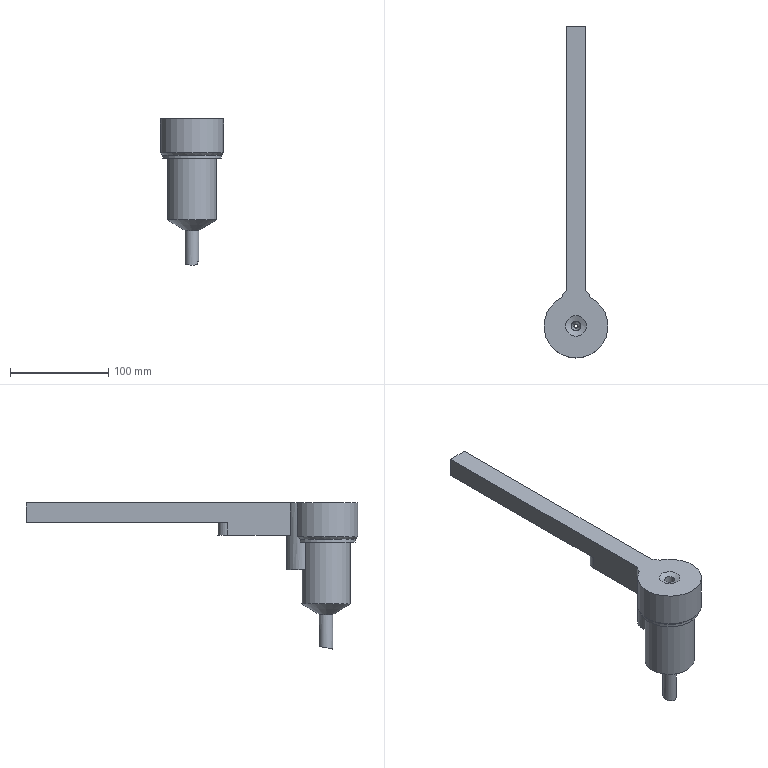Part | STEP file | 车灯-后视镜_id722_x_t | 1 solid | 26 faces | box 65 x 337.5 x 148.701 mm | volume 402158 mm3 | plane 11 | cylinder 7 | cone 4 | sphere 2 | spline 1 | other 1 | commonest cylinder face diameters 10 x1 14 x1 20 x1 30 x1 50 x1 60 x1
STEP:
#1=CARTESIAN_POINT('',(-29.,-25.,97.005));
#2=VERTEX_POINT('',#1);
#3=CARTESIAN_POINT('',(-22.,-25.,97.005));
#4=DIRECTION('',(0.,0.,1.));
#5=DIRECTION('',(-1.,0.,0.));
#6=AXIS2_PLACEMENT_3D('',#3,#4,#5);
#7=CIRCLE('',#6,7.);
#8=EDGE_CURVE('',#2,#2,#7,.T.);
#9=ORIENTED_EDGE('',*,*,#8,.F.);
#10=EDGE_LOOP('',(#9));
#11=FACE_BOUND('',#10,.T.);
#12=CARTESIAN_POINT('',(-15.953,-28.525,62.553));
#13=VERTEX_POINT('',#12);
#14=CARTESIAN_POINT('',(-15.953,-21.475,64.005));
#15=VERTEX_POINT('',#14);
#16=CARTESIAN_POINT('',(-15.953,-28.525,62.553));
#17=CARTESIAN_POINT('',(-16.721,-29.844,62.271));
#18=CARTESIAN_POINT('',(-17.908,-30.885,62.044));
#19=CARTESIAN_POINT('',(-20.758,-32.059,61.786));
#20=CARTESIAN_POINT('',(-22.363,-32.159,61.764));
#21=CARTESIAN_POINT('',(-25.338,-31.343,61.943));
#22=CARTESIAN_POINT('',(-26.657,-30.443,62.141));
#23=CARTESIAN_POINT('',(-28.497,-28.018,62.662));
#24=CARTESIAN_POINT('',(-28.997,-26.523,62.978));
#25=CARTESIAN_POINT('',(-29.003,-23.51,63.598));
#26=CARTESIAN_POINT('',(-28.503,-22.001,63.901));
#27=CARTESIAN_POINT('',(-26.683,-19.581,64.379));
#28=CARTESIAN_POINT('',(-25.346,-18.664,64.556));
#29=CARTESIAN_POINT('',(-22.399,-17.846,64.714));
#30=CARTESIAN_POINT('',(-20.766,-17.942,64.696));
#31=CARTESIAN_POINT('',(-17.938,-19.098,64.472));
#32=CARTESIAN_POINT('',(-16.723,-20.153,64.268));
#33=CARTESIAN_POINT('',(-15.953,-21.475,64.005));
#34=B_SPLINE_CURVE_WITH_KNOTS('',3,(#16,#17,#18,#19,#20,#21,#22,#23,#24,#25,#26,#27,#28,#29,#30,#31,#32,#33),.UNSPECIFIED.,.F.,.F.,(4,2,2,2,2,2,2,2,4),(0.,0.125,0.25,0.375,0.5,0.625,0.75,0.875,1.),.UNSPECIFIED.);
#35=EDGE_CURVE('',#13,#15,#34,.T.);
#36=ORIENTED_EDGE('',*,*,#35,.F.);
#37=CARTESIAN_POINT('',(-15.953,-28.525,65.088));
#38=VERTEX_POINT('',#37);
#39=CARTESIAN_POINT('',(-15.953,-28.525,63.319));
#40=DIRECTION('',(0.,0.,-1.));
#41=VECTOR('',#40,1.);
#42=LINE('',#39,#41);
#43=EDGE_CURVE('',#38,#13,#42,.T.);
#44=ORIENTED_EDGE('',*,*,#43,.F.);
#45=CARTESIAN_POINT('',(-15.953,-21.475,66.533));
#46=VERTEX_POINT('',#45);
#47=CARTESIAN_POINT('',(-15.953,-21.475,66.533));
#48=CARTESIAN_POINT('',(-15.349,-22.51,66.163));
#49=CARTESIAN_POINT('',(-15.009,-23.717,65.827));
#50=CARTESIAN_POINT('',(-14.991,-26.184,65.317));
#51=CARTESIAN_POINT('',(-15.322,-27.443,65.144));
#52=CARTESIAN_POINT('',(-15.953,-28.525,65.088));
#53=B_SPLINE_CURVE_WITH_KNOTS('',3,(#47,#48,#49,#50,#51,#52),.UNSPECIFIED.,.F.,.F.,(4,2,4),(0.,0.5,1.),.UNSPECIFIED.);
#54=EDGE_CURVE('',#46,#38,#53,.T.);
#55=ORIENTED_EDGE('',*,*,#54,.F.);
#56=CARTESIAN_POINT('',(-15.953,-21.475,63.897));
#57=DIRECTION('',(0.,0.,1.));
#58=VECTOR('',#57,1.);
#59=LINE('',#56,#58);
#60=EDGE_CURVE('',#15,#46,#59,.T.);
#61=ORIENTED_EDGE('',*,*,#60,.F.);
#62=EDGE_LOOP('',(#36,#44,#55,#61));
#63=FACE_BOUND('',#62,.T.);
#64=CARTESIAN_POINT('',(-22.,-25.,107.82));
#65=DIRECTION('',(0.,0.,-1.));
#66=DIRECTION('',(1.,0.,0.));
#67=AXIS2_PLACEMENT_3D('',#64,#65,#66);
#68=CYLINDRICAL_SURFACE('',#67,7.);
#69=ADVANCED_FACE('',(#11,#63),#68,.T.);
#70=CARTESIAN_POINT('',(-23.499,-25.,121.));
#71=VERTEX_POINT('',#70);
#72=CARTESIAN_POINT('',(-22.,-25.,121.));
#73=DIRECTION('',(0.,0.,-1.));
#74=DIRECTION('',(-1.,0.,0.));
#75=AXIS2_PLACEMENT_3D('',#72,#73,#74);
#76=CIRCLE('',#75,1.499);
#77=EDGE_CURVE('',#71,#71,#76,.T.);
#78=ORIENTED_EDGE('',*,*,#77,.F.);
#79=EDGE_LOOP('',(#78));
#80=FACE_BOUND('',#79,.T.);
#81=CARTESIAN_POINT('',(-18.452,-27.856,62.695));
#82=VERTEX_POINT('',#81);
#83=CARTESIAN_POINT('',(-18.517,-22.162,63.868));
#84=VERTEX_POINT('',#83);
#85=CARTESIAN_POINT('',(-18.452,-27.856,62.695));
#86=CARTESIAN_POINT('',(-19.029,-28.587,62.54));
#87=CARTESIAN_POINT('',(-19.826,-29.126,62.424));
#88=CARTESIAN_POINT('',(-21.62,-29.654,62.311));
#89=CARTESIAN_POINT('',(-22.603,-29.63,62.316));
#90=CARTESIAN_POINT('',(-24.362,-29.019,62.447));
#91=CARTESIAN_POINT('',(-25.144,-28.43,62.573));
#92=CARTESIAN_POINT('',(-26.213,-26.937,62.889));
#93=CARTESIAN_POINT('',(-26.512,-26.018,63.082));
#94=CARTESIAN_POINT('',(-26.546,-23.28,63.646));
#95=CARTESIAN_POINT('',(-25.348,-21.473,64.006));
#96=CARTESIAN_POINT('',(-21.834,-20.152,64.266));
#97=CARTESIAN_POINT('',(-19.708,-20.724,64.156));
#98=CARTESIAN_POINT('',(-18.517,-22.162,63.868));
#99=B_SPLINE_CURVE_WITH_KNOTS('',3,(#85,#86,#87,#88,#89,#90,#91,#92,#93,#94,#95,#96,#97,#98),.UNSPECIFIED.,.F.,.F.,(4,2,2,2,2,2,4),(0.,0.125,0.25,0.375,0.5,0.75,1.),.UNSPECIFIED.);
#100=EDGE_CURVE('',#82,#84,#99,.T.);
#101=ORIENTED_EDGE('',*,*,#100,.T.);
#102=CARTESIAN_POINT('',(-18.699,-22.21,67.137));
#103=VERTEX_POINT('',#102);
#104=CARTESIAN_POINT('',(-18.517,-22.162,63.868));
#105=CARTESIAN_POINT('',(-18.577,-22.178,64.957));
#106=CARTESIAN_POINT('',(-18.638,-22.194,66.047));
#107=CARTESIAN_POINT('',(-18.699,-22.21,67.137));
#108=B_SPLINE_CURVE_WITH_KNOTS('',3,(#104,#105,#106,#107),.UNSPECIFIED.,.F.,.F.,(4,4),(0.,1.),.UNSPECIFIED.);
#109=EDGE_CURVE('',#84,#103,#108,.T.);
#110=ORIENTED_EDGE('',*,*,#109,.T.);
#111=CARTESIAN_POINT('',(-18.634,-27.807,65.974));
#112=VERTEX_POINT('',#111);
#113=CARTESIAN_POINT('',(-18.699,-22.21,67.137));
#114=CARTESIAN_POINT('',(-18.051,-22.95,66.813));
#115=CARTESIAN_POINT('',(-17.657,-23.933,66.507));
#116=CARTESIAN_POINT('',(-17.611,-25.962,66.079));
#117=CARTESIAN_POINT('',(-17.964,-27.006,65.959));
#118=CARTESIAN_POINT('',(-18.634,-27.807,65.974));
#119=B_SPLINE_CURVE_WITH_KNOTS('',3,(#113,#114,#115,#116,#117,#118),.UNSPECIFIED.,.F.,.F.,(4,2,4),(0.,0.5,1.),.UNSPECIFIED.);
#120=EDGE_CURVE('',#103,#112,#119,.T.);
#121=ORIENTED_EDGE('',*,*,#120,.T.);
#122=CARTESIAN_POINT('',(-18.634,-27.807,65.974));
#123=CARTESIAN_POINT('',(-18.573,-27.823,64.881));
#124=CARTESIAN_POINT('',(-18.512,-27.84,63.788));
#125=CARTESIAN_POINT('',(-18.452,-27.856,62.695));
#126=B_SPLINE_CURVE_WITH_KNOTS('',3,(#122,#123,#124,#125),.UNSPECIFIED.,.F.,.F.,(4,4),(0.,1.),.UNSPECIFIED.);
#127=EDGE_CURVE('',#112,#82,#126,.T.);
#128=ORIENTED_EDGE('',*,*,#127,.T.);
#129=EDGE_LOOP('',(#101,#110,#121,#128));
#130=FACE_BOUND('',#129,.T.);
#131=CARTESIAN_POINT('',(-22.,-25.,120.974));
#132=DIRECTION('',(0.,0.,-1.));
#133=DIRECTION('',(1.,0.,0.));
#134=AXIS2_PLACEMENT_3D('',#131,#132,#133);
#135=CONICAL_SURFACE('',#134,1.501,3.);
#136=ADVANCED_FACE('',(#80,#130),#135,.F.);
#137=CARTESIAN_POINT('',(-12.,75.,190.5));
#138=VERTEX_POINT('',#137);
#139=CARTESIAN_POINT('',(-32.,75.,190.5));
#140=VERTEX_POINT('',#139);
#141=CARTESIAN_POINT('',(-22.,75.,190.5));
#142=DIRECTION('',(0.,0.,1.));
#143=DIRECTION('',(1.,0.,0.));
#144=AXIS2_PLACEMENT_3D('',#141,#142,#143);
#145=CIRCLE('',#144,10.);
#146=EDGE_CURVE('',#138,#140,#145,.T.);
#147=ORIENTED_EDGE('',*,*,#146,.T.);
#148=CARTESIAN_POINT('',(-32.,280.,190.5));
#149=VERTEX_POINT('',#148);
#150=CARTESIAN_POINT('',(-32.,11.18,190.5));
#151=DIRECTION('',(0.,-1.,0.));
#152=VECTOR('',#151,1.);
#153=LINE('',#150,#152);
#154=EDGE_CURVE('',#149,#140,#153,.T.);
#155=ORIENTED_EDGE('',*,*,#154,.F.);
#156=CARTESIAN_POINT('',(-12.,280.,190.5));
#157=VERTEX_POINT('',#156);
#158=CARTESIAN_POINT('',(3.,280.,190.5));
#159=DIRECTION('',(-1.,0.,0.));
#160=VECTOR('',#159,1.);
#161=LINE('',#158,#160);
#162=EDGE_CURVE('',#157,#149,#161,.T.);
#163=ORIENTED_EDGE('',*,*,#162,.F.);
#164=CARTESIAN_POINT('',(-12.,0.,190.5));
#165=DIRECTION('',(0.,-1.,0.));
#166=VECTOR('',#165,1.);
#167=LINE('',#164,#166);
#168=EDGE_CURVE('',#157,#138,#167,.T.);
#169=ORIENTED_EDGE('',*,*,#168,.T.);
#170=EDGE_LOOP('',(#147,#155,#163,#169));
#171=FACE_OUTER_BOUND('',#170,.T.);
#172=CARTESIAN_POINT('',(-22.,0.,190.5));
#173=DIRECTION('',(0.,0.,1.));
#174=DIRECTION('',(0.,-1.,0.));
#175=AXIS2_PLACEMENT_3D('',#172,#173,#174);
#176=PLANE('',#175);
#177=ADVANCED_FACE('',(#171),#176,.F.);
#178=CARTESIAN_POINT('',(-12.,11.18,210.5));
#179=VERTEX_POINT('',#178);
#180=CARTESIAN_POINT('',(-12.,280.,210.5));
#181=VERTEX_POINT('',#180);
#182=CARTESIAN_POINT('',(-12.,11.18,210.5));
#183=DIRECTION('',(0.,1.,0.));
#184=VECTOR('',#183,1.);
#185=LINE('',#182,#184);
#186=EDGE_CURVE('',#179,#181,#185,.T.);
#187=ORIENTED_EDGE('',*,*,#186,.T.);
#188=CARTESIAN_POINT('',(-32.,280.,210.5));
#189=VERTEX_POINT('',#188);
#190=CARTESIAN_POINT('',(3.,280.,210.5));
#191=DIRECTION('',(-1.,0.,0.));
#192=VECTOR('',#191,1.);
#193=LINE('',#190,#192);
#194=EDGE_CURVE('',#181,#189,#193,.T.);
#195=ORIENTED_EDGE('',*,*,#194,.T.);
#196=CARTESIAN_POINT('',(-32.,11.18,210.5));
#197=VERTEX_POINT('',#196);
#198=CARTESIAN_POINT('',(-32.,-25.,210.5));
#199=DIRECTION('',(0.,-1.,0.));
#200=VECTOR('',#199,1.);
#201=LINE('',#198,#200);
#202=EDGE_CURVE('',#189,#197,#201,.T.);
#203=ORIENTED_EDGE('',*,*,#202,.T.);
#204=CARTESIAN_POINT('',(-36.422,4.125,210.5));
#205=VERTEX_POINT('',#204);
#206=CARTESIAN_POINT('',(-22.,0.,210.5));
#207=DIRECTION('',(0.,0.,1.));
#208=DIRECTION('',(1.,0.,0.));
#209=AXIS2_PLACEMENT_3D('',#206,#207,#208);
#210=CIRCLE('',#209,15.);
#211=EDGE_CURVE('',#197,#205,#210,.T.);
#212=ORIENTED_EDGE('',*,*,#211,.T.);
#213=CARTESIAN_POINT('',(-7.578,4.125,210.5));
#214=VERTEX_POINT('',#213);
#215=CARTESIAN_POINT('',(-22.,-25.,210.5));
#216=DIRECTION('',(0.,0.,1.));
#217=DIRECTION('',(1.,0.,0.));
#218=AXIS2_PLACEMENT_3D('',#215,#216,#217);
#219=CIRCLE('',#218,32.5);
#220=EDGE_CURVE('',#205,#214,#219,.T.);
#221=ORIENTED_EDGE('',*,*,#220,.T.);
#222=CARTESIAN_POINT('',(-22.,0.,210.5));
#223=DIRECTION('',(0.,0.,1.));
#224=DIRECTION('',(1.,0.,0.));
#225=AXIS2_PLACEMENT_3D('',#222,#223,#224);
#226=CIRCLE('',#225,15.);
#227=EDGE_CURVE('',#214,#179,#226,.T.);
#228=ORIENTED_EDGE('',*,*,#227,.T.);
#229=EDGE_LOOP('',(#187,#195,#203,#212,#221,#228));
#230=FACE_BOUND('',#229,.T.);
#231=CARTESIAN_POINT('',(-11.464,-25.,210.5));
#232=VERTEX_POINT('',#231);
#233=CARTESIAN_POINT('',(-22.,-25.,210.5));
#234=DIRECTION('',(0.,0.,1.));
#235=DIRECTION('',(1.,0.,0.));
#236=AXIS2_PLACEMENT_3D('',#233,#234,#235);
#237=CIRCLE('',#236,10.536);
#238=EDGE_CURVE('',#232,#232,#237,.T.);
#239=ORIENTED_EDGE('',*,*,#238,.F.);
#240=EDGE_LOOP('',(#239));
#241=FACE_BOUND('',#240,.T.);
#242=CARTESIAN_POINT('',(-22.,-25.,210.5));
#243=DIRECTION('',(0.,0.,1.));
#244=DIRECTION('',(0.,-1.,0.));
#245=AXIS2_PLACEMENT_3D('',#242,#243,#244);
#246=PLANE('',#245);
#247=ADVANCED_FACE('',(#230,#241),#246,.T.);
#248=ORIENTED_EDGE('',*,*,#168,.F.);
#249=CARTESIAN_POINT('',(-12.,280.,0.5));
#250=DIRECTION('',(0.,0.,-1.));
#251=VECTOR('',#250,1.);
#252=LINE('',#249,#251);
#253=EDGE_CURVE('',#181,#157,#252,.T.);
#254=ORIENTED_EDGE('',*,*,#253,.F.);
#255=ORIENTED_EDGE('',*,*,#186,.F.);
#256=CARTESIAN_POINT('',(-12.,11.18,177.5));
#257=VERTEX_POINT('',#256);
#258=CARTESIAN_POINT('',(-12.,11.18,142.5));
#259=DIRECTION('',(0.,0.,1.));
#260=VECTOR('',#259,1.);
#261=LINE('',#258,#260);
#262=EDGE_CURVE('',#257,#179,#261,.T.);
#263=ORIENTED_EDGE('',*,*,#262,.F.);
#264=CARTESIAN_POINT('',(-12.,75.,177.5));
#265=VERTEX_POINT('',#264);
#266=CARTESIAN_POINT('',(-12.,11.18,177.5));
#267=DIRECTION('',(0.,1.,0.));
#268=VECTOR('',#267,1.);
#269=LINE('',#266,#268);
#270=EDGE_CURVE('',#257,#265,#269,.T.);
#271=ORIENTED_EDGE('',*,*,#270,.T.);
#272=CARTESIAN_POINT('',(-12.,75.,162.5));
#273=DIRECTION('',(0.,0.,-1.));
#274=VECTOR('',#273,1.);
#275=LINE('',#272,#274);
#276=EDGE_CURVE('',#138,#265,#275,.T.);
#277=ORIENTED_EDGE('',*,*,#276,.F.);
#278=EDGE_LOOP('',(#248,#254,#255,#263,#271,#277));
#279=FACE_OUTER_BOUND('',#278,.T.);
#280=CARTESIAN_POINT('',(-12.,11.18,172.5));
#281=DIRECTION('',(-1.,0.,0.));
#282=DIRECTION('',(0.,0.,-1.));
#283=AXIS2_PLACEMENT_3D('',#280,#281,#282);
#284=PLANE('',#283);
#285=ADVANCED_FACE('',(#279),#284,.F.);
#286=CARTESIAN_POINT('',(-32.,11.18,177.5));
#287=VERTEX_POINT('',#286);
#288=CARTESIAN_POINT('',(-22.,0.,177.5));
#289=DIRECTION('',(0.,0.,-1.));
#290=DIRECTION('',(1.,0.,0.));
#291=AXIS2_PLACEMENT_3D('',#288,#289,#290);
#292=CIRCLE('',#291,15.);
#293=EDGE_CURVE('',#287,#257,#292,.T.);
#294=ORIENTED_EDGE('',*,*,#293,.F.);
#295=CARTESIAN_POINT('',(-32.,75.,177.5));
#296=VERTEX_POINT('',#295);
#297=CARTESIAN_POINT('',(-32.,11.18,177.5));
#298=DIRECTION('',(0.,1.,0.));
#299=VECTOR('',#298,1.);
#300=LINE('',#297,#299);
#301=EDGE_CURVE('',#287,#296,#300,.T.);
#302=ORIENTED_EDGE('',*,*,#301,.T.);
#303=CARTESIAN_POINT('',(-22.,75.,177.5));
#304=DIRECTION('',(0.,0.,1.));
#305=DIRECTION('',(1.,0.,0.));
#306=AXIS2_PLACEMENT_3D('',#303,#304,#305);
#307=CIRCLE('',#306,10.);
#308=EDGE_CURVE('',#265,#296,#307,.T.);
#309=ORIENTED_EDGE('',*,*,#308,.F.);
#310=ORIENTED_EDGE('',*,*,#270,.F.);
#311=EDGE_LOOP('',(#294,#302,#309,#310));
#312=FACE_OUTER_BOUND('',#311,.T.);
#313=CARTESIAN_POINT('',(-22.,75.,177.5));
#314=DIRECTION('',(0.,0.,1.));
#315=DIRECTION('',(-1.,0.,0.));
#316=AXIS2_PLACEMENT_3D('',#313,#314,#315);
#317=PLANE('',#316);
#318=ADVANCED_FACE('',(#312),#317,.F.);
#319=CARTESIAN_POINT('',(3.,-25.,107.82));
#320=VERTEX_POINT('',#319);
#321=CARTESIAN_POINT('',(-22.,-25.,107.82));
#322=DIRECTION('',(0.,0.,1.));
#323=DIRECTION('',(1.,0.,0.));
#324=AXIS2_PLACEMENT_3D('',#321,#322,#323);
#325=CIRCLE('',#324,25.);
#326=EDGE_CURVE('',#320,#320,#325,.T.);
#327=ORIENTED_EDGE('',*,*,#326,.T.);
#328=EDGE_LOOP('',(#327));
#329=FACE_BOUND('',#328,.T.);
#330=CARTESIAN_POINT('',(-7.691,-4.5,170.5));
#331=VERTEX_POINT('',#330);
#332=CARTESIAN_POINT('',(-36.309,-4.5,170.5));
#333=VERTEX_POINT('',#332);
#334=CARTESIAN_POINT('',(-22.,-25.,170.5));
#335=DIRECTION('',(0.,0.,-1.));
#336=DIRECTION('',(-1.,0.,0.));
#337=AXIS2_PLACEMENT_3D('',#334,#335,#336);
#338=CIRCLE('',#337,25.);
#339=EDGE_CURVE('',#331,#333,#338,.T.);
#340=ORIENTED_EDGE('',*,*,#339,.T.);
#341=CARTESIAN_POINT('',(-36.309,-4.5,142.5));
#342=VERTEX_POINT('',#341);
#343=CARTESIAN_POINT('',(-36.309,-4.5,142.5));
#344=DIRECTION('',(0.,0.,1.));
#345=VECTOR('',#344,1.);
#346=LINE('',#343,#345);
#347=EDGE_CURVE('',#342,#333,#346,.T.);
#348=ORIENTED_EDGE('',*,*,#347,.F.);
#349=CARTESIAN_POINT('',(-7.691,-4.5,142.5));
#350=VERTEX_POINT('',#349);
#351=CARTESIAN_POINT('',(-22.,-25.,142.5));
#352=DIRECTION('',(0.,0.,-1.));
#353=DIRECTION('',(1.,0.,0.));
#354=AXIS2_PLACEMENT_3D('',#351,#352,#353);
#355=CIRCLE('',#354,25.);
#356=EDGE_CURVE('',#342,#350,#355,.T.);
#357=ORIENTED_EDGE('',*,*,#356,.T.);
#358=CARTESIAN_POINT('',(-7.691,-4.5,-145.68));
#359=DIRECTION('',(0.,0.,-1.));
#360=VECTOR('',#359,1.);
#361=LINE('',#358,#360);
#362=EDGE_CURVE('',#331,#350,#361,.T.);
#363=ORIENTED_EDGE('',*,*,#362,.F.);
#364=EDGE_LOOP('',(#340,#348,#357,#363));
#365=FACE_BOUND('',#364,.T.);
#366=CARTESIAN_POINT('',(-22.,-25.,-145.68));
#367=DIRECTION('',(0.,0.,1.));
#368=DIRECTION('',(-1.,0.,0.));
#369=AXIS2_PLACEMENT_3D('',#366,#367,#368);
#370=CYLINDRICAL_SURFACE('',#369,25.);
#371=ADVANCED_FACE('',(#329,#365),#370,.T.);
#372=CARTESIAN_POINT('',(-22.,0.,142.5));
#373=DIRECTION('',(0.,0.,-1.));
#374=DIRECTION('',(1.,0.,0.));
#375=AXIS2_PLACEMENT_3D('',#372,#373,#374);
#376=CIRCLE('',#375,15.);
#377=EDGE_CURVE('',#342,#350,#376,.T.);
#378=ORIENTED_EDGE('',*,*,#377,.F.);
#379=ORIENTED_EDGE('',*,*,#347,.T.);
#380=CARTESIAN_POINT('',(-36.967,1.,170.5));
#381=VERTEX_POINT('',#380);
#382=CARTESIAN_POINT('',(-22.,0.,170.5));
#383=DIRECTION('',(0.,0.,-1.));
#384=DIRECTION('',(-1.,0.,0.));
#385=AXIS2_PLACEMENT_3D('',#382,#383,#384);
#386=CIRCLE('',#385,15.);
#387=EDGE_CURVE('',#333,#381,#386,.T.);
#388=ORIENTED_EDGE('',*,*,#387,.T.);
#389=CARTESIAN_POINT('',(-36.967,1.,173.5));
#390=VERTEX_POINT('',#389);
#391=CARTESIAN_POINT('',(-36.967,1.,186.5));
#392=DIRECTION('',(0.,0.,1.));
#393=VECTOR('',#392,1.);
#394=LINE('',#391,#393);
#395=EDGE_CURVE('',#381,#390,#394,.T.);
#396=ORIENTED_EDGE('',*,*,#395,.T.);
#397=CARTESIAN_POINT('',(-36.422,4.125,176.));
#398=VERTEX_POINT('',#397);
#399=CARTESIAN_POINT('',(-36.967,1.,173.5));
#400=CARTESIAN_POINT('',(-36.932,1.518,173.931));
#401=CARTESIAN_POINT('',(-36.87,2.042,174.359));
#402=CARTESIAN_POINT('',(-36.689,3.085,175.193));
#403=CARTESIAN_POINT('',(-36.57,3.606,175.601));
#404=CARTESIAN_POINT('',(-36.422,4.125,176.));
#405=B_SPLINE_CURVE_WITH_KNOTS('',3,(#399,#400,#401,#402,#403,#404),.UNSPECIFIED.,.F.,.F.,(4,2,4),(0.,0.5,1.),.UNSPECIFIED.);
#406=EDGE_CURVE('',#390,#398,#405,.T.);
#407=ORIENTED_EDGE('',*,*,#406,.T.);
#408=CARTESIAN_POINT('',(-36.422,4.125,186.5));
#409=DIRECTION('',(0.,0.,1.));
#410=VECTOR('',#409,1.);
#411=LINE('',#408,#410);
#412=EDGE_CURVE('',#398,#205,#411,.T.);
#413=ORIENTED_EDGE('',*,*,#412,.T.);
#414=ORIENTED_EDGE('',*,*,#211,.F.);
#415=CARTESIAN_POINT('',(-32.,11.18,142.5));
#416=DIRECTION('',(0.,0.,1.));
#417=VECTOR('',#416,1.);
#418=LINE('',#415,#417);
#419=EDGE_CURVE('',#287,#197,#418,.T.);
#420=ORIENTED_EDGE('',*,*,#419,.F.);
#421=ORIENTED_EDGE('',*,*,#293,.T.);
#422=ORIENTED_EDGE('',*,*,#262,.T.);
#423=ORIENTED_EDGE('',*,*,#227,.F.);
#424=CARTESIAN_POINT('',(-7.578,4.125,176.));
#425=VERTEX_POINT('',#424);
#426=CARTESIAN_POINT('',(-7.578,4.125,186.5));
#427=DIRECTION('',(0.,0.,-1.));
#428=VECTOR('',#427,1.);
#429=LINE('',#426,#428);
#430=EDGE_CURVE('',#214,#425,#429,.T.);
#431=ORIENTED_EDGE('',*,*,#430,.T.);
#432=CARTESIAN_POINT('',(-7.033,1.,173.5));
#433=VERTEX_POINT('',#432);
#434=CARTESIAN_POINT('',(-7.578,4.125,176.));
#435=CARTESIAN_POINT('',(-7.43,3.606,175.601));
#436=CARTESIAN_POINT('',(-7.311,3.085,175.192));
#437=CARTESIAN_POINT('',(-7.129,2.037,174.355));
#438=CARTESIAN_POINT('',(-7.068,1.514,173.929));
#439=CARTESIAN_POINT('',(-7.033,1.,173.5));
#440=B_SPLINE_CURVE_WITH_KNOTS('',3,(#434,#435,#436,#437,#438,#439),.UNSPECIFIED.,.F.,.F.,(4,2,4),(0.,0.5,1.),.UNSPECIFIED.);
#441=EDGE_CURVE('',#425,#433,#440,.T.);
#442=ORIENTED_EDGE('',*,*,#441,.T.);
#443=CARTESIAN_POINT('',(-7.033,1.,170.5));
#444=VERTEX_POINT('',#443);
#445=CARTESIAN_POINT('',(-7.033,1.,186.5));
#446=DIRECTION('',(0.,0.,-1.));
#447=VECTOR('',#446,1.);
#448=LINE('',#445,#447);
#449=EDGE_CURVE('',#433,#444,#448,.T.);
#450=ORIENTED_EDGE('',*,*,#449,.T.);
#451=CARTESIAN_POINT('',(-22.,0.,170.5));
#452=DIRECTION('',(0.,0.,-1.));
#453=DIRECTION('',(-1.,0.,0.));
#454=AXIS2_PLACEMENT_3D('',#451,#452,#453);
#455=CIRCLE('',#454,15.);
#456=EDGE_CURVE('',#444,#331,#455,.T.);
#457=ORIENTED_EDGE('',*,*,#456,.T.);
#458=ORIENTED_EDGE('',*,*,#362,.T.);
#459=EDGE_LOOP('',(#378,#379,#388,#396,#407,#413,#414,#420,#421,#422,#423,#431,#442,#450,#457,#458));
#460=FACE_OUTER_BOUND('',#459,.T.);
#461=CARTESIAN_POINT('',(-22.,0.,142.5));
#462=DIRECTION('',(0.,0.,1.));
#463=DIRECTION('',(-1.,0.,0.));
#464=AXIS2_PLACEMENT_3D('',#461,#462,#463);
#465=CYLINDRICAL_SURFACE('',#464,15.);
#466=ADVANCED_FACE('',(#460),#465,.T.);
#467=ORIENTED_EDGE('',*,*,#356,.F.);
#468=ORIENTED_EDGE('',*,*,#377,.T.);
#469=EDGE_LOOP('',(#467,#468));
#470=FACE_OUTER_BOUND('',#469,.T.);
#471=CARTESIAN_POINT('',(-19.,-12.5,142.5));
#472=DIRECTION('',(0.,0.,1.));
#473=DIRECTION('',(-1.,0.,0.));
#474=AXIS2_PLACEMENT_3D('',#471,#472,#473);
#475=PLANE('',#474);
#476=ADVANCED_FACE('',(#470),#475,.F.);
#477=ORIENTED_EDGE('',*,*,#8,.T.);
#478=EDGE_LOOP('',(#477));
#479=FACE_BOUND('',#478,.T.);
#480=ORIENTED_EDGE('',*,*,#326,.F.);
#481=EDGE_LOOP('',(#480));
#482=FACE_BOUND('',#481,.T.);
#483=CARTESIAN_POINT('',(-22.,-25.,92.798));
#484=DIRECTION('',(0.,0.,1.));
#485=DIRECTION('',(-1.,0.,0.));
#486=AXIS2_PLACEMENT_3D('',#483,#484,#485);
#487=CONICAL_SURFACE('',#486,0.,59.);
#488=ADVANCED_FACE('',(#479,#482),#487,.T.);
#489=ORIENTED_EDGE('',*,*,#220,.F.);
#490=ORIENTED_EDGE('',*,*,#412,.F.);
#491=CARTESIAN_POINT('',(-22.,-25.,176.));
#492=DIRECTION('',(0.,0.,1.));
#493=DIRECTION('',(1.,0.,0.));
#494=AXIS2_PLACEMENT_3D('',#491,#492,#493);
#495=CIRCLE('',#494,32.5);
#496=EDGE_CURVE('',#398,#425,#495,.T.);
#497=ORIENTED_EDGE('',*,*,#496,.T.);
#498=ORIENTED_EDGE('',*,*,#430,.F.);
#499=EDGE_LOOP('',(#489,#490,#497,#498));
#500=FACE_OUTER_BOUND('',#499,.T.);
#501=CARTESIAN_POINT('',(-22.,-25.,210.5));
#502=DIRECTION('',(0.,0.,-1.));
#503=DIRECTION('',(1.,0.,0.));
#504=AXIS2_PLACEMENT_3D('',#501,#502,#503);
#505=CYLINDRICAL_SURFACE('',#504,32.5);
#506=ADVANCED_FACE('',(#500),#505,.T.);
#507=ORIENTED_EDGE('',*,*,#496,.F.);
#508=ORIENTED_EDGE('',*,*,#406,.F.);
#509=CARTESIAN_POINT('',(-22.,-25.,173.5));
#510=DIRECTION('',(0.,0.,1.));
#511=DIRECTION('',(-1.,0.,0.));
#512=AXIS2_PLACEMENT_3D('',#509,#510,#511);
#513=CIRCLE('',#512,30.);
#514=EDGE_CURVE('',#390,#433,#513,.T.);
#515=ORIENTED_EDGE('',*,*,#514,.T.);
#516=ORIENTED_EDGE('',*,*,#441,.F.);
#517=EDGE_LOOP('',(#507,#508,#515,#516));
#518=FACE_OUTER_BOUND('',#517,.T.);
#519=CARTESIAN_POINT('',(-22.,-25.,176.));
#520=DIRECTION('',(0.,0.,1.));
#521=DIRECTION('',(1.,0.,0.));
#522=AXIS2_PLACEMENT_3D('',#519,#520,#521);
#523=CONICAL_SURFACE('',#522,32.5,45.);
#524=ADVANCED_FACE('',(#518),#523,.T.);
#525=ORIENTED_EDGE('',*,*,#514,.F.);
#526=ORIENTED_EDGE('',*,*,#395,.F.);
#527=CARTESIAN_POINT('',(-22.,-25.,170.5));
#528=DIRECTION('',(0.,0.,-1.));
#529=DIRECTION('',(-1.,0.,0.));
#530=AXIS2_PLACEMENT_3D('',#527,#528,#529);
#531=CIRCLE('',#530,30.);
#532=EDGE_CURVE('',#444,#381,#531,.T.);
#533=ORIENTED_EDGE('',*,*,#532,.F.);
#534=ORIENTED_EDGE('',*,*,#449,.F.);
#535=EDGE_LOOP('',(#525,#526,#533,#534));
#536=FACE_OUTER_BOUND('',#535,.T.);
#537=CARTESIAN_POINT('',(-22.,-25.,176.));
#538=DIRECTION('',(0.,0.,-1.));
#539=DIRECTION('',(1.,0.,0.));
#540=AXIS2_PLACEMENT_3D('',#537,#538,#539);
#541=CYLINDRICAL_SURFACE('',#540,30.);
#542=ADVANCED_FACE('',(#536),#541,.T.);
#543=ORIENTED_EDGE('',*,*,#532,.T.);
#544=ORIENTED_EDGE('',*,*,#387,.F.);
#545=ORIENTED_EDGE('',*,*,#339,.F.);
#546=ORIENTED_EDGE('',*,*,#456,.F.);
#547=EDGE_LOOP('',(#543,#544,#545,#546));
#548=FACE_OUTER_BOUND('',#547,.T.);
#549=CARTESIAN_POINT('',(-22.,-25.,170.5));
#550=DIRECTION('',(0.,0.,-1.));
#551=DIRECTION('',(1.,0.,0.));
#552=AXIS2_PLACEMENT_3D('',#549,#550,#551);
#553=PLANE('',#552);
#554=ADVANCED_FACE('',(#548),#553,.T.);
#555=ORIENTED_EDGE('',*,*,#308,.T.);
#556=CARTESIAN_POINT('',(-32.,75.,172.5));
#557=DIRECTION('',(0.,0.,1.));
#558=VECTOR('',#557,1.);
#559=LINE('',#556,#558);
#560=EDGE_CURVE('',#296,#140,#559,.T.);
#561=ORIENTED_EDGE('',*,*,#560,.T.);
#562=ORIENTED_EDGE('',*,*,#146,.F.);
#563=ORIENTED_EDGE('',*,*,#276,.T.);
#564=EDGE_LOOP('',(#555,#561,#562,#563));
#565=FACE_OUTER_BOUND('',#564,.T.);
#566=CARTESIAN_POINT('',(-22.,75.,172.5));
#567=DIRECTION('',(0.,0.,-1.));
#568=DIRECTION('',(0.,1.,0.));
#569=AXIS2_PLACEMENT_3D('',#566,#567,#568);
#570=CYLINDRICAL_SURFACE('',#569,10.);
#571=ADVANCED_FACE('',(#565),#570,.T.);
#572=ORIENTED_EDGE('',*,*,#238,.T.);
#573=EDGE_LOOP('',(#572));
#574=FACE_BOUND('',#573,.T.);
#575=CARTESIAN_POINT('',(-17.,-25.,208.135));
#576=VERTEX_POINT('',#575);
#577=CARTESIAN_POINT('',(-22.,-25.,208.135));
#578=DIRECTION('',(0.,0.,1.));
#579=DIRECTION('',(1.,0.,0.));
#580=AXIS2_PLACEMENT_3D('',#577,#578,#579);
#581=CIRCLE('',#580,5.);
#582=EDGE_CURVE('',#576,#576,#581,.T.);
#583=ORIENTED_EDGE('',*,*,#582,.F.);
#584=EDGE_LOOP('',(#583));
#585=FACE_BOUND('',#584,.T.);
#586=CARTESIAN_POINT('',(-22.,-25.,227.5));
#587=DIRECTION('',(0.,0.,1.));
#588=DIRECTION('',(1.,0.,0.));
#589=AXIS2_PLACEMENT_3D('',#586,#587,#588);
#590=SPHERICAL_SURFACE('',#589,20.);
#591=ADVANCED_FACE('',(#574,#585),#590,.F.);
#592=CARTESIAN_POINT('',(-19.599,-25.,121.));
#593=VERTEX_POINT('',#592);
#594=CARTESIAN_POINT('',(-22.,-25.,121.));
#595=DIRECTION('',(0.,0.,-1.));
#596=DIRECTION('',(1.,0.,0.));
#597=AXIS2_PLACEMENT_3D('',#594,#595,#596);
#598=CIRCLE('',#597,2.401);
#599=EDGE_CURVE('',#593,#593,#598,.T.);
#600=ORIENTED_EDGE('',*,*,#599,.F.);
#601=EDGE_LOOP('',(#600));
#602=FACE_BOUND('',#601,.T.);
#603=ORIENTED_EDGE('',*,*,#77,.T.);
#604=EDGE_LOOP('',(#603));
#605=FACE_BOUND('',#604,.T.);
#606=CARTESIAN_POINT('',(-22.,-25.,121.));
#607=DIRECTION('',(0.,0.,-1.));
#608=DIRECTION('',(1.,0.,0.));
#609=AXIS2_PLACEMENT_3D('',#606,#607,#608);
#610=PLANE('',#609);
#611=ADVANCED_FACE('',(#602,#605),#610,.F.);
#612=ORIENTED_EDGE('',*,*,#202,.F.);
#613=CARTESIAN_POINT('',(-32.,280.,0.5));
#614=DIRECTION('',(0.,0.,-1.));
#615=VECTOR('',#614,1.);
#616=LINE('',#613,#615);
#617=EDGE_CURVE('',#189,#149,#616,.T.);
#618=ORIENTED_EDGE('',*,*,#617,.T.);
#619=ORIENTED_EDGE('',*,*,#154,.T.);
#620=ORIENTED_EDGE('',*,*,#560,.F.);
#621=ORIENTED_EDGE('',*,*,#301,.F.);
#622=ORIENTED_EDGE('',*,*,#419,.T.);
#623=EDGE_LOOP('',(#612,#618,#619,#620,#621,#622));
#624=FACE_OUTER_BOUND('',#623,.T.);
#625=CARTESIAN_POINT('',(-32.,11.18,172.5));
#626=DIRECTION('',(-1.,0.,0.));
#627=DIRECTION('',(0.,1.,0.));
#628=AXIS2_PLACEMENT_3D('',#625,#626,#627);
#629=PLANE('',#628);
#630=ADVANCED_FACE('',(#624),#629,.T.);
#631=CARTESIAN_POINT('',(-27.,-25.,129.792));
#632=VERTEX_POINT('',#631);
#633=CARTESIAN_POINT('',(-22.,-25.,129.792));
#634=DIRECTION('',(0.,0.,1.));
#635=DIRECTION('',(-1.,0.,0.));
#636=AXIS2_PLACEMENT_3D('',#633,#634,#635);
#637=CIRCLE('',#636,5.);
#638=EDGE_CURVE('',#632,#632,#637,.T.);
#639=ORIENTED_EDGE('',*,*,#638,.F.);
#640=EDGE_LOOP('',(#639));
#641=FACE_BOUND('',#640,.T.);
#642=ORIENTED_EDGE('',*,*,#582,.T.);
#643=EDGE_LOOP('',(#642));
#644=FACE_BOUND('',#643,.T.);
#645=CARTESIAN_POINT('',(-22.,-25.,99.5));
#646=DIRECTION('',(0.,0.,1.));
#647=DIRECTION('',(-1.,0.,0.));
#648=AXIS2_PLACEMENT_3D('',#645,#646,#647);
#649=CYLINDRICAL_SURFACE('',#648,5.);
#650=ADVANCED_FACE('',(#641,#644),#649,.F.);
#651=CARTESIAN_POINT('',(-26.755,-25.,128.247));
#652=VERTEX_POINT('',#651);
#653=CARTESIAN_POINT('',(-22.,-25.,128.247));
#654=DIRECTION('',(0.,0.,-1.));
#655=DIRECTION('',(-1.,0.,0.));
#656=AXIS2_PLACEMENT_3D('',#653,#654,#655);
#657=CIRCLE('',#656,4.755);
#658=EDGE_CURVE('',#652,#652,#657,.T.);
#659=ORIENTED_EDGE('',*,*,#658,.F.);
#660=EDGE_LOOP('',(#659));
#661=FACE_BOUND('',#660,.T.);
#662=ORIENTED_EDGE('',*,*,#599,.T.);
#663=EDGE_LOOP('',(#662));
#664=FACE_BOUND('',#663,.T.);
#665=CARTESIAN_POINT('',(-22.,-25.,129.));
#666=DIRECTION('',(0.,0.,1.));
#667=DIRECTION('',(-1.,0.,0.));
#668=AXIS2_PLACEMENT_3D('',#665,#666,#667);
#669=CONICAL_SURFACE('',#668,5.,18.);
#670=ADVANCED_FACE('',(#661,#664),#669,.F.);
#671=ORIENTED_EDGE('',*,*,#638,.T.);
#672=EDGE_LOOP('',(#671));
#673=FACE_BOUND('',#672,.T.);
#674=ORIENTED_EDGE('',*,*,#658,.T.);
#675=EDGE_LOOP('',(#674));
#676=FACE_BOUND('',#675,.T.);
#677=CARTESIAN_POINT('',(-22.,-25.,129.792));
#678=DIRECTION('',(0.,0.,1.));
#679=DIRECTION('',(-1.,0.,0.));
#680=AXIS2_PLACEMENT_3D('',#677,#678,#679);
#681=SPHERICAL_SURFACE('',#680,5.);
#682=ADVANCED_FACE('',(#673,#676),#681,.F.);
#683=ORIENTED_EDGE('',*,*,#253,.T.);
#684=ORIENTED_EDGE('',*,*,#162,.T.);
#685=ORIENTED_EDGE('',*,*,#617,.F.);
#686=ORIENTED_EDGE('',*,*,#194,.F.);
#687=EDGE_LOOP('',(#683,#684,#685,#686));
#688=FACE_OUTER_BOUND('',#687,.T.);
#689=CARTESIAN_POINT('',(3.,280.,0.5));
#690=DIRECTION('',(0.,1.,0.));
#691=DIRECTION('',(0.,0.,1.));
#692=AXIS2_PLACEMENT_3D('',#689,#690,#691);
#693=PLANE('',#692);
#694=ADVANCED_FACE('',(#688),#693,.T.);
#695=ORIENTED_EDGE('',*,*,#43,.T.);
#696=CARTESIAN_POINT('',(-18.452,-27.856,62.695));
#697=CARTESIAN_POINT('',(-17.619,-28.079,62.648));
#698=CARTESIAN_POINT('',(-16.786,-28.302,62.6));
#699=CARTESIAN_POINT('',(-15.953,-28.525,62.553));
#700=B_SPLINE_CURVE_WITH_KNOTS('',3,(#696,#697,#698,#699),.UNSPECIFIED.,.F.,.F.,(4,4),(0.,1.),.UNSPECIFIED.);
#701=EDGE_CURVE('',#82,#13,#700,.T.);
#702=ORIENTED_EDGE('',*,*,#701,.F.);
#703=ORIENTED_EDGE('',*,*,#127,.F.);
#704=CARTESIAN_POINT('',(-15.953,-28.525,65.088));
#705=CARTESIAN_POINT('',(-16.846,-28.286,65.383));
#706=CARTESIAN_POINT('',(-17.74,-28.047,65.678));
#707=CARTESIAN_POINT('',(-18.634,-27.807,65.974));
#708=B_SPLINE_CURVE_WITH_KNOTS('',3,(#704,#705,#706,#707),.UNSPECIFIED.,.F.,.F.,(4,4),(0.,1.),.UNSPECIFIED.);
#709=EDGE_CURVE('',#38,#112,#708,.T.);
#710=ORIENTED_EDGE('',*,*,#709,.F.);
#711=EDGE_LOOP('',(#695,#702,#703,#710));
#712=FACE_OUTER_BOUND('',#711,.T.);
#713=CARTESIAN_POINT('',(-12.316,-29.5,61.427));
#714=DIRECTION('',(-0.2588,-0.9659,0.));
#715=DIRECTION('',(0.9659,-0.2588,0.));
#716=AXIS2_PLACEMENT_3D('',#713,#714,#715);
#717=PLANE('',#716);
#718=ADVANCED_FACE('',(#712),#717,.F.);
#719=ORIENTED_EDGE('',*,*,#54,.T.);
#720=ORIENTED_EDGE('',*,*,#709,.T.);
#721=ORIENTED_EDGE('',*,*,#120,.F.);
#722=CARTESIAN_POINT('',(-18.699,-22.21,67.137));
#723=CARTESIAN_POINT('',(-17.783,-21.965,66.936));
#724=CARTESIAN_POINT('',(-16.868,-21.72,66.734));
#725=CARTESIAN_POINT('',(-15.953,-21.475,66.533));
#726=B_SPLINE_CURVE_WITH_KNOTS('',3,(#722,#723,#724,#725),.UNSPECIFIED.,.F.,.F.,(4,4),(0.,1.),.UNSPECIFIED.);
#727=EDGE_CURVE('',#103,#46,#726,.T.);
#728=ORIENTED_EDGE('',*,*,#727,.T.);
#729=EDGE_LOOP('',(#719,#720,#721,#728));
#730=FACE_OUTER_BOUND('',#729,.T.);
#731=CARTESIAN_POINT('',(-21.316,36.979,76.906));
#732=CARTESIAN_POINT('',(-21.316,22.634,75.233));
#733=CARTESIAN_POINT('',(-21.316,8.315,73.269));
#734=CARTESIAN_POINT('',(-21.316,-20.212,68.418));
#735=CARTESIAN_POINT('',(-21.316,-34.398,65.517));
#736=CARTESIAN_POINT('',(-21.316,-48.448,61.901));
#737=CARTESIAN_POINT('',(-9.316,37.352,73.712));
#738=CARTESIAN_POINT('',(-9.316,23.052,72.045));
#739=CARTESIAN_POINT('',(-9.316,8.785,70.087));
#740=CARTESIAN_POINT('',(-9.316,-19.603,65.26));
#741=CARTESIAN_POINT('',(-9.316,-33.7,62.376));
#742=CARTESIAN_POINT('',(-9.316,-47.646,58.787));
#743=B_SPLINE_SURFACE_WITH_KNOTS('',1,3,((#731,#732,#733,#734,#735,#736),(#737,#738,#739,#740,#741,#742)),.UNSPECIFIED.,.F.,.F.,.F.,(2,2),(4,2,4),(0.,1.),(0.,0.5,1.),.UNSPECIFIED.);
#744=ADVANCED_FACE('',(#730),#743,.T.);
#745=ORIENTED_EDGE('',*,*,#60,.T.);
#746=ORIENTED_EDGE('',*,*,#727,.F.);
#747=ORIENTED_EDGE('',*,*,#109,.F.);
#748=CARTESIAN_POINT('',(-15.953,-21.475,64.005));
#749=CARTESIAN_POINT('',(-16.807,-21.704,63.959));
#750=CARTESIAN_POINT('',(-17.662,-21.933,63.914));
#751=CARTESIAN_POINT('',(-18.517,-22.162,63.868));
#752=B_SPLINE_CURVE_WITH_KNOTS('',3,(#748,#749,#750,#751),.UNSPECIFIED.,.F.,.F.,(4,4),(0.,1.),.UNSPECIFIED.);
#753=EDGE_CURVE('',#15,#84,#752,.T.);
#754=ORIENTED_EDGE('',*,*,#753,.F.);
#755=EDGE_LOOP('',(#745,#746,#747,#754));
#756=FACE_OUTER_BOUND('',#755,.T.);
#757=CARTESIAN_POINT('',(-12.316,-20.5,62.147));
#758=DIRECTION('',(-0.2588,0.9659,0.));
#759=DIRECTION('',(-0.9659,-0.2588,0.));
#760=AXIS2_PLACEMENT_3D('',#757,#758,#759);
#761=PLANE('',#760);
#762=ADVANCED_FACE('',(#756),#761,.F.);
#763=ORIENTED_EDGE('',*,*,#701,.T.);
#764=ORIENTED_EDGE('',*,*,#35,.T.);
#765=ORIENTED_EDGE('',*,*,#753,.T.);
#766=ORIENTED_EDGE('',*,*,#100,.F.);
#767=EDGE_LOOP('',(#763,#764,#765,#766));
#768=FACE_OUTER_BOUND('',#767,.T.);
#769=CARTESIAN_POINT('',(-12.332,37.444,73.018));
#770=CARTESIAN_POINT('',(-12.381,30.166,72.169));
#771=CARTESIAN_POINT('',(-12.445,22.978,71.252));
#772=CARTESIAN_POINT('',(-12.521,15.838,70.249));
#773=CARTESIAN_POINT('',(-12.596,8.698,69.246));
#774=CARTESIAN_POINT('',(-12.683,1.606,68.157));
#775=CARTESIAN_POINT('',(-12.783,-5.456,66.954));
#776=CARTESIAN_POINT('',(-12.883,-12.518,65.751));
#777=CARTESIAN_POINT('',(-12.995,-19.549,64.434));
#778=CARTESIAN_POINT('',(-13.126,-26.549,62.97));
#779=CARTESIAN_POINT('',(-13.256,-33.549,61.506));
#780=CARTESIAN_POINT('',(-13.404,-40.518,59.896));
#781=CARTESIAN_POINT('',(-13.579,-47.447,58.113));
#782=B_SPLINE_CURVE_WITH_KNOTS('',3,(#769,#770,#771,#772,#773,#774,#775,#776,#777,#778,#779,#780,#781),.UNSPECIFIED.,.F.,.F.,(4,3,3,3,4),(0.,0.25,0.5,0.75,1.),.UNSPECIFIED.);
#783=DIRECTION('',(-1.,0.,0.));
#784=VECTOR('',#783,1.);
#785=SURFACE_OF_LINEAR_EXTRUSION('',#782,#784);
#786=ADVANCED_FACE('',(#768),#785,.T.);
#787=CLOSED_SHELL('',(#69,#136,#177,#247,#285,#318,#371,#466,#476,#488,#506,#524,#542,#554,#571,#591,#611,#630,#650,#670,#682,#694,#718,#744,#762,#786));
#788=MANIFOLD_SOLID_BREP('',#787);
#789=(LENGTH_UNIT()NAMED_UNIT(*)SI_UNIT(.MILLI.,.METRE.));
#790=UNCERTAINTY_MEASURE_WITH_UNIT(LENGTH_MEASURE(0.0508),#789,'','');
#791=(NAMED_UNIT(*)PLANE_ANGLE_UNIT()SI_UNIT($,.RADIAN.));
#792=PLANE_ANGLE_MEASURE_WITH_UNIT(PLANE_ANGLE_MEASURE(0.01745),#791);
#793=DIMENSIONAL_EXPONENTS(0.,0.,0.,0.,0.,0.,0.);
#794=(CONVERSION_BASED_UNIT('DEGREE',#792)NAMED_UNIT(#793)PLANE_ANGLE_UNIT());
#795=(NAMED_UNIT(*)SI_UNIT($,.STERADIAN.)SOLID_ANGLE_UNIT());
#796=(GEOMETRIC_REPRESENTATION_CONTEXT(3)GLOBAL_UNCERTAINTY_ASSIGNED_CONTEXT((#790))GLOBAL_UNIT_ASSIGNED_CONTEXT((#789,#794,#795))REPRESENTATION_CONTEXT('',''));
#797=ADVANCED_BREP_SHAPE_REPRESENTATION('',(#788),#796);